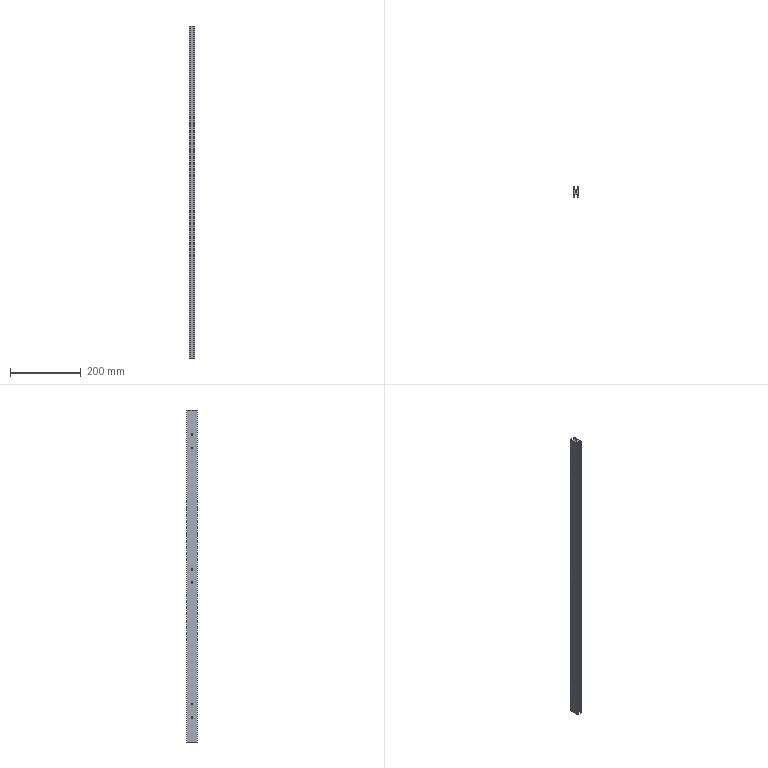Part | SolidWorks | features BaseBody 1 | 1 solid | 68 faces | box 15 x 30 x 936 mm | volume 262278 mm3 | cylinder 38 | plane 30 | commonest cylinder face diameters 5 x38